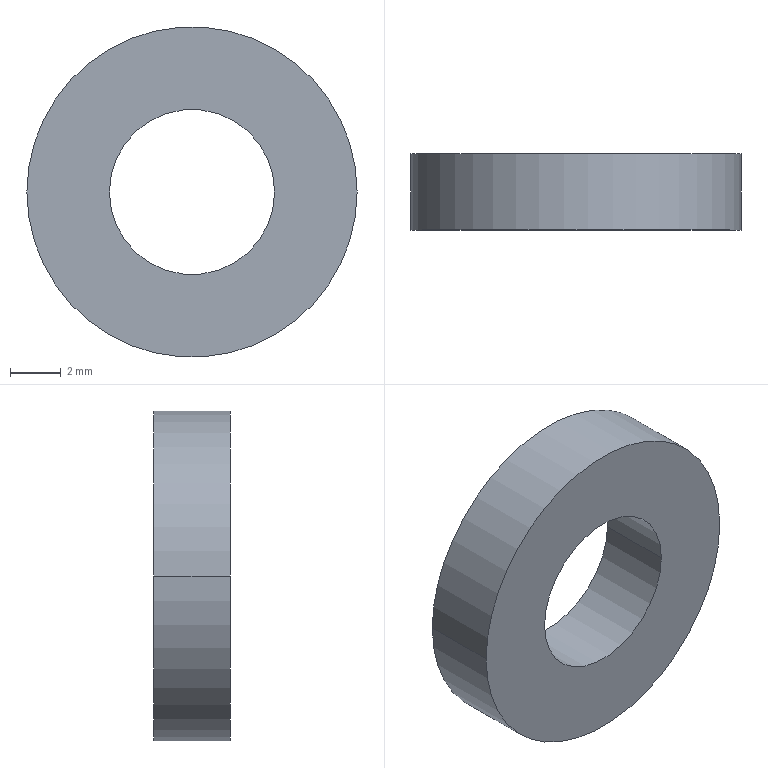Part | STEP file | WSX-SUS-M6X13-3 | 1 solid | 6 faces | box 13 x 3 x 13 mm | volume 298.648 mm3 | cylinder 4 | plane 2 | commonest cylinder face diameters 6.5 x2 13 x2
STEP:
#1=CARTESIAN_POINT('',(3.25,3.,0.));
#2=VERTEX_POINT('',#1);
#3=CARTESIAN_POINT('',(-3.25,3.,0.));
#4=VERTEX_POINT('',#3);
#5=CARTESIAN_POINT('',(0.,3.,0.));
#6=DIRECTION('',(0.,-1.,0.));
#7=DIRECTION('',(-1.,0.,0.));
#8=AXIS2_PLACEMENT_3D('',#5,#6,#7);
#9=CIRCLE('',#8,3.25);
#10=EDGE_CURVE('',#2,#4,#9,.T.);
#11=ORIENTED_EDGE('',*,*,#10,.F.);
#12=CARTESIAN_POINT('',(3.25,0.,0.));
#13=VERTEX_POINT('',#12);
#14=CARTESIAN_POINT('',(3.25,3.,0.));
#15=DIRECTION('',(0.,-1.,0.));
#16=VECTOR('',#15,1000.);
#17=LINE('',#14,#16);
#18=EDGE_CURVE('',#2,#13,#17,.T.);
#19=ORIENTED_EDGE('',*,*,#18,.T.);
#20=CARTESIAN_POINT('',(-3.25,0.,0.));
#21=VERTEX_POINT('',#20);
#22=CARTESIAN_POINT('',(0.,0.,0.));
#23=DIRECTION('',(0.,1.,0.));
#24=DIRECTION('',(1.,0.,0.));
#25=AXIS2_PLACEMENT_3D('',#22,#23,#24);
#26=CIRCLE('',#25,3.25);
#27=EDGE_CURVE('',#21,#13,#26,.T.);
#28=ORIENTED_EDGE('',*,*,#27,.F.);
#29=CARTESIAN_POINT('',(-3.25,3.,0.));
#30=DIRECTION('',(0.,-1.,0.));
#31=VECTOR('',#30,1000.);
#32=LINE('',#29,#31);
#33=EDGE_CURVE('',#4,#21,#32,.T.);
#34=ORIENTED_EDGE('',*,*,#33,.F.);
#35=EDGE_LOOP('',(#11,#19,#28,#34));
#36=FACE_OUTER_BOUND('',#35,.T.);
#37=CARTESIAN_POINT('',(0.,3.,0.));
#38=DIRECTION('',(0.,-1.,0.));
#39=DIRECTION('',(-1.,0.,0.));
#40=AXIS2_PLACEMENT_3D('',#37,#38,#39);
#41=CYLINDRICAL_SURFACE('',#40,3.25);
#42=ADVANCED_FACE('',(#36),#41,.F.);
#43=CARTESIAN_POINT('',(-6.5,3.,0.));
#44=VERTEX_POINT('',#43);
#45=CARTESIAN_POINT('',(6.5,3.,0.));
#46=VERTEX_POINT('',#45);
#47=CARTESIAN_POINT('',(0.,3.,0.));
#48=DIRECTION('',(0.,-1.,0.));
#49=DIRECTION('',(-1.,0.,0.));
#50=AXIS2_PLACEMENT_3D('',#47,#48,#49);
#51=CIRCLE('',#50,6.5);
#52=EDGE_CURVE('',#44,#46,#51,.T.);
#53=ORIENTED_EDGE('',*,*,#52,.T.);
#54=CARTESIAN_POINT('',(6.5,0.,0.));
#55=VERTEX_POINT('',#54);
#56=CARTESIAN_POINT('',(6.5,3.,0.));
#57=DIRECTION('',(0.,-1.,0.));
#58=VECTOR('',#57,1000.);
#59=LINE('',#56,#58);
#60=EDGE_CURVE('',#46,#55,#59,.T.);
#61=ORIENTED_EDGE('',*,*,#60,.T.);
#62=CARTESIAN_POINT('',(-6.5,0.,0.));
#63=VERTEX_POINT('',#62);
#64=CARTESIAN_POINT('',(0.,0.,0.));
#65=DIRECTION('',(0.,1.,0.));
#66=DIRECTION('',(1.,0.,0.));
#67=AXIS2_PLACEMENT_3D('',#64,#65,#66);
#68=CIRCLE('',#67,6.5);
#69=EDGE_CURVE('',#55,#63,#68,.T.);
#70=ORIENTED_EDGE('',*,*,#69,.T.);
#71=CARTESIAN_POINT('',(-6.5,3.,0.));
#72=DIRECTION('',(0.,-1.,0.));
#73=VECTOR('',#72,1000.);
#74=LINE('',#71,#73);
#75=EDGE_CURVE('',#44,#63,#74,.T.);
#76=ORIENTED_EDGE('',*,*,#75,.F.);
#77=EDGE_LOOP('',(#53,#61,#70,#76));
#78=FACE_OUTER_BOUND('',#77,.T.);
#79=CARTESIAN_POINT('',(0.,3.,0.));
#80=DIRECTION('',(0.,-1.,0.));
#81=DIRECTION('',(-1.,0.,0.));
#82=AXIS2_PLACEMENT_3D('',#79,#80,#81);
#83=CYLINDRICAL_SURFACE('',#82,6.5);
#84=ADVANCED_FACE('',(#78),#83,.T.);
#85=ORIENTED_EDGE('',*,*,#27,.T.);
#86=CARTESIAN_POINT('',(0.,0.,0.));
#87=DIRECTION('',(0.,1.,0.));
#88=DIRECTION('',(1.,0.,0.));
#89=AXIS2_PLACEMENT_3D('',#86,#87,#88);
#90=CIRCLE('',#89,3.25);
#91=EDGE_CURVE('',#13,#21,#90,.T.);
#92=ORIENTED_EDGE('',*,*,#91,.T.);
#93=EDGE_LOOP('',(#85,#92));
#94=FACE_BOUND('',#93,.T.);
#95=CARTESIAN_POINT('',(0.,0.,0.));
#96=DIRECTION('',(0.,1.,0.));
#97=DIRECTION('',(1.,0.,0.));
#98=AXIS2_PLACEMENT_3D('',#95,#96,#97);
#99=CIRCLE('',#98,6.5);
#100=EDGE_CURVE('',#63,#55,#99,.T.);
#101=ORIENTED_EDGE('',*,*,#100,.F.);
#102=ORIENTED_EDGE('',*,*,#69,.F.);
#103=EDGE_LOOP('',(#101,#102));
#104=FACE_OUTER_BOUND('',#103,.T.);
#105=CARTESIAN_POINT('',(0.,0.,0.));
#106=DIRECTION('',(0.,-1.,0.));
#107=DIRECTION('',(-1.,0.,0.));
#108=AXIS2_PLACEMENT_3D('',#105,#106,#107);
#109=PLANE('',#108);
#110=ADVANCED_FACE('',(#94,#104),#109,.T.);
#111=CARTESIAN_POINT('',(0.,3.,0.));
#112=DIRECTION('',(0.,-1.,0.));
#113=DIRECTION('',(-1.,0.,0.));
#114=AXIS2_PLACEMENT_3D('',#111,#112,#113);
#115=CIRCLE('',#114,3.25);
#116=EDGE_CURVE('',#4,#2,#115,.T.);
#117=ORIENTED_EDGE('',*,*,#116,.T.);
#118=ORIENTED_EDGE('',*,*,#10,.T.);
#119=EDGE_LOOP('',(#117,#118));
#120=FACE_BOUND('',#119,.T.);
#121=ORIENTED_EDGE('',*,*,#52,.F.);
#122=CARTESIAN_POINT('',(0.,3.,0.));
#123=DIRECTION('',(0.,-1.,0.));
#124=DIRECTION('',(-1.,0.,0.));
#125=AXIS2_PLACEMENT_3D('',#122,#123,#124);
#126=CIRCLE('',#125,6.5);
#127=EDGE_CURVE('',#46,#44,#126,.T.);
#128=ORIENTED_EDGE('',*,*,#127,.F.);
#129=EDGE_LOOP('',(#121,#128));
#130=FACE_OUTER_BOUND('',#129,.T.);
#131=CARTESIAN_POINT('',(0.,3.,0.));
#132=DIRECTION('',(0.,1.,0.));
#133=DIRECTION('',(1.,0.,0.));
#134=AXIS2_PLACEMENT_3D('',#131,#132,#133);
#135=PLANE('',#134);
#136=ADVANCED_FACE('',(#120,#130),#135,.T.);
#137=ORIENTED_EDGE('',*,*,#60,.F.);
#138=ORIENTED_EDGE('',*,*,#127,.T.);
#139=ORIENTED_EDGE('',*,*,#75,.T.);
#140=ORIENTED_EDGE('',*,*,#100,.T.);
#141=EDGE_LOOP('',(#137,#138,#139,#140));
#142=FACE_OUTER_BOUND('',#141,.T.);
#143=CARTESIAN_POINT('',(0.,3.,0.));
#144=DIRECTION('',(0.,-1.,0.));
#145=DIRECTION('',(-1.,0.,0.));
#146=AXIS2_PLACEMENT_3D('',#143,#144,#145);
#147=CYLINDRICAL_SURFACE('',#146,6.5);
#148=ADVANCED_FACE('',(#142),#147,.T.);
#149=ORIENTED_EDGE('',*,*,#18,.F.);
#150=ORIENTED_EDGE('',*,*,#116,.F.);
#151=ORIENTED_EDGE('',*,*,#33,.T.);
#152=ORIENTED_EDGE('',*,*,#91,.F.);
#153=EDGE_LOOP('',(#149,#150,#151,#152));
#154=FACE_OUTER_BOUND('',#153,.T.);
#155=CARTESIAN_POINT('',(0.,3.,0.));
#156=DIRECTION('',(0.,-1.,0.));
#157=DIRECTION('',(-1.,0.,0.));
#158=AXIS2_PLACEMENT_3D('',#155,#156,#157);
#159=CYLINDRICAL_SURFACE('',#158,3.25);
#160=ADVANCED_FACE('',(#154),#159,.F.);
#161=CLOSED_SHELL('',(#42,#84,#110,#136,#148,#160));
#162=MANIFOLD_SOLID_BREP('',#161);
#163=CARTESIAN_POINT('',(0.,0.,0.));
#164=DIRECTION('',(0.,0.,1.));
#165=DIRECTION('',(1.,0.,0.));
#166=AXIS2_PLACEMENT_3D('',#163,#164,#165);
#167=(LENGTH_UNIT()NAMED_UNIT(*)SI_UNIT(.MILLI.,.METRE.));
#168=UNCERTAINTY_MEASURE_WITH_UNIT(LENGTH_MEASURE(0.00001),#167,'','');
#169=(NAMED_UNIT(*)PLANE_ANGLE_UNIT()SI_UNIT($,.RADIAN.));
#170=(NAMED_UNIT(*)SI_UNIT($,.STERADIAN.)SOLID_ANGLE_UNIT());
#171=(GEOMETRIC_REPRESENTATION_CONTEXT(3)GLOBAL_UNCERTAINTY_ASSIGNED_CONTEXT((#168))GLOBAL_UNIT_ASSIGNED_CONTEXT((#167,#169,#170))REPRESENTATION_CONTEXT('',''));
#172=ADVANCED_BREP_SHAPE_REPRESENTATION('',(#162,#166),#171);